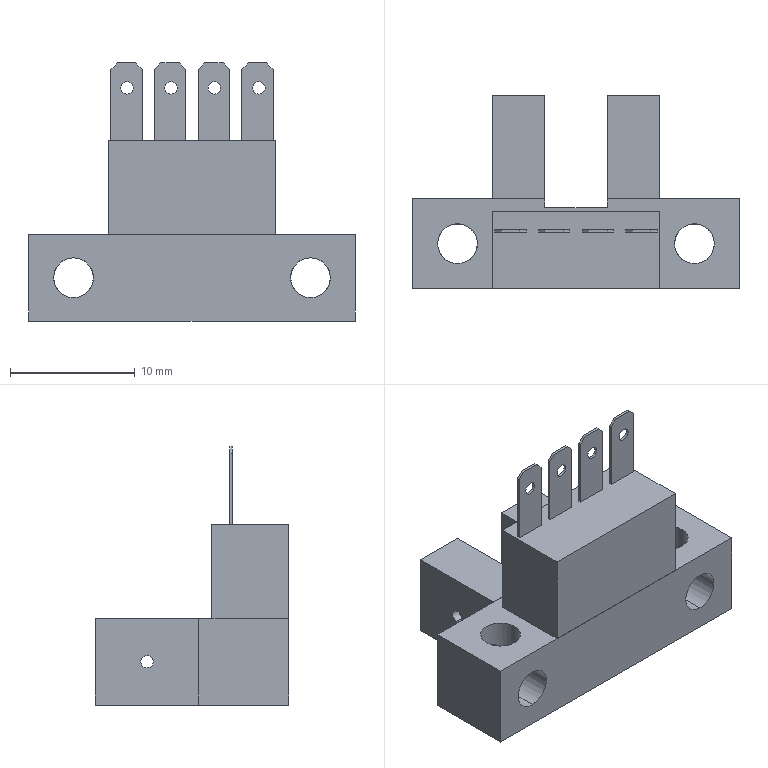Part | STEP file | EE-SX671 (sensing SENSORS) | 1 solid | 79 faces | box 26.2 x 15.5 x 20.7 mm | volume 2220 mm3 | plane 51 | cylinder 28 | commonest cylinder face diameters 3.2 x16 1 x12